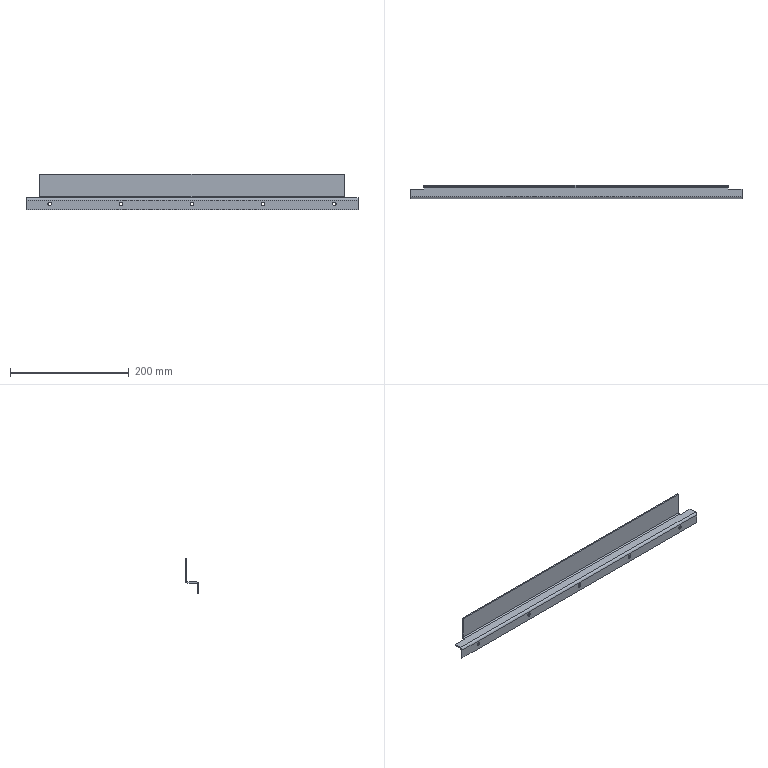Part | NX | features solid 2 | 1 solid | 28 faces | box 560 x 22 x 60 mm | volume 82302 mm3 | plane 14 | cylinder 14 | commonest cylinder face diameters 6 x10 4 x2 8 x2
STEP:
#1=CARTESIAN_POINT('',(1859.9,-1560.,278.));
#2=VERTEX_POINT('',#1);
#3=CARTESIAN_POINT('',(1859.9,-1562.,278.));
#4=VERTEX_POINT('',#3);
#5=CARTESIAN_POINT('',(1859.9,-1578.,278.));
#6=DIRECTION('',(0.,-1.,0.));
#7=VECTOR('',#6,1000.);
#8=LINE('',#5,#7);
#9=EDGE_CURVE('',#2,#4,#8,.T.);
#10=ORIENTED_EDGE('',*,*,#9,.F.);
#11=CARTESIAN_POINT('',(1859.9,-1556.,282.));
#12=VERTEX_POINT('',#11);
#13=CARTESIAN_POINT('',(1859.9,-1560.,282.));
#14=DIRECTION('',(-1.,0.,0.));
#15=DIRECTION('',(0.,0.,-1.));
#16=AXIS2_PLACEMENT_3D('',#13,#14,#15);
#17=CIRCLE('',#16,4.);
#18=EDGE_CURVE('',#12,#2,#17,.T.);
#19=ORIENTED_EDGE('',*,*,#18,.F.);
#20=CARTESIAN_POINT('',(1859.9,-1556.,320.));
#21=VERTEX_POINT('',#20);
#22=CARTESIAN_POINT('',(1859.9,-1556.,280.));
#23=DIRECTION('',(0.,0.,-1.));
#24=VECTOR('',#23,1000.);
#25=LINE('',#22,#24);
#26=EDGE_CURVE('',#21,#12,#25,.T.);
#27=ORIENTED_EDGE('',*,*,#26,.F.);
#28=CARTESIAN_POINT('',(1859.9,-1558.,320.));
#29=VERTEX_POINT('',#28);
#30=CARTESIAN_POINT('',(1859.9,-1558.,320.));
#31=DIRECTION('',(0.,-1.,0.));
#32=VECTOR('',#31,1000.);
#33=LINE('',#30,#32);
#34=EDGE_CURVE('',#21,#29,#33,.T.);
#35=ORIENTED_EDGE('',*,*,#34,.T.);
#36=CARTESIAN_POINT('',(1859.9,-1558.,282.));
#37=VERTEX_POINT('',#36);
#38=CARTESIAN_POINT('',(1859.9,-1558.,280.));
#39=DIRECTION('',(0.,0.,-1.));
#40=VECTOR('',#39,1000.);
#41=LINE('',#38,#40);
#42=EDGE_CURVE('',#29,#37,#41,.T.);
#43=ORIENTED_EDGE('',*,*,#42,.T.);
#44=CARTESIAN_POINT('',(1859.9,-1560.,280.));
#45=VERTEX_POINT('',#44);
#46=CARTESIAN_POINT('',(1859.9,-1560.,282.));
#47=DIRECTION('',(-1.,0.,0.));
#48=DIRECTION('',(0.,0.,-1.));
#49=AXIS2_PLACEMENT_3D('',#46,#47,#48);
#50=CIRCLE('',#49,2.);
#51=EDGE_CURVE('',#37,#45,#50,.T.);
#52=ORIENTED_EDGE('',*,*,#51,.T.);
#53=CARTESIAN_POINT('',(1859.9,-1562.,280.));
#54=VERTEX_POINT('',#53);
#55=CARTESIAN_POINT('',(1859.9,-1578.,280.));
#56=DIRECTION('',(0.,-1.,0.));
#57=VECTOR('',#56,1000.);
#58=LINE('',#55,#57);
#59=EDGE_CURVE('',#45,#54,#58,.T.);
#60=ORIENTED_EDGE('',*,*,#59,.T.);
#61=CARTESIAN_POINT('',(1859.9,-1562.,280.));
#62=DIRECTION('',(0.,0.,1.));
#63=VECTOR('',#62,1000.);
#64=LINE('',#61,#63);
#65=EDGE_CURVE('',#4,#54,#64,.T.);
#66=ORIENTED_EDGE('',*,*,#65,.F.);
#67=EDGE_LOOP('',(#10,#19,#27,#35,#43,#52,#60,#66));
#68=FACE_BOUND('',#67,.T.);
#69=CARTESIAN_POINT('',(1859.9,-1578.,280.));
#70=DIRECTION('',(-1.,0.,0.));
#71=DIRECTION('',(0.,0.,1.));
#72=AXIS2_PLACEMENT_3D('',#69,#70,#71);
#73=PLANE('',#72);
#74=ADVANCED_FACE('',(#68),#73,.F.);
#75=ORIENTED_EDGE('',*,*,#65,.T.);
#76=CARTESIAN_POINT('',(1883.,-1562.,280.));
#77=VERTEX_POINT('',#76);
#78=CARTESIAN_POINT('',(1883.,-1562.,280.));
#79=DIRECTION('',(-1.,0.,0.));
#80=VECTOR('',#79,1000.);
#81=LINE('',#78,#80);
#82=EDGE_CURVE('',#77,#54,#81,.T.);
#83=ORIENTED_EDGE('',*,*,#82,.F.);
#84=CARTESIAN_POINT('',(1883.,-1562.,278.));
#85=VERTEX_POINT('',#84);
#86=CARTESIAN_POINT('',(1883.,-1562.,280.));
#87=DIRECTION('',(0.,0.,1.));
#88=VECTOR('',#87,1000.);
#89=LINE('',#86,#88);
#90=EDGE_CURVE('',#85,#77,#89,.T.);
#91=ORIENTED_EDGE('',*,*,#90,.F.);
#92=CARTESIAN_POINT('',(1883.,-1562.,278.));
#93=DIRECTION('',(-1.,0.,0.));
#94=VECTOR('',#93,1000.);
#95=LINE('',#92,#94);
#96=EDGE_CURVE('',#85,#4,#95,.T.);
#97=ORIENTED_EDGE('',*,*,#96,.T.);
#98=EDGE_LOOP('',(#75,#83,#91,#97));
#99=FACE_BOUND('',#98,.T.);
#100=CARTESIAN_POINT('',(1883.,-1562.,280.));
#101=DIRECTION('',(0.,1.,0.));
#102=DIRECTION('',(0.,0.,-1.));
#103=AXIS2_PLACEMENT_3D('',#100,#101,#102);
#104=PLANE('',#103);
#105=ADVANCED_FACE('',(#99),#104,.T.);
#106=CARTESIAN_POINT('',(1346.1,-1556.,282.));
#107=VERTEX_POINT('',#106);
#108=CARTESIAN_POINT('',(1346.1,-1556.,320.));
#109=VERTEX_POINT('',#108);
#110=CARTESIAN_POINT('',(1346.1,-1556.,280.));
#111=DIRECTION('',(0.,0.,1.));
#112=VECTOR('',#111,1000.);
#113=LINE('',#110,#112);
#114=EDGE_CURVE('',#107,#109,#113,.T.);
#115=ORIENTED_EDGE('',*,*,#114,.F.);
#116=CARTESIAN_POINT('',(1346.1,-1560.,278.));
#117=VERTEX_POINT('',#116);
#118=CARTESIAN_POINT('',(1346.1,-1560.,282.));
#119=DIRECTION('',(1.,0.,0.));
#120=DIRECTION('',(0.,0.,-1.));
#121=AXIS2_PLACEMENT_3D('',#118,#119,#120);
#122=CIRCLE('',#121,4.);
#123=EDGE_CURVE('',#117,#107,#122,.T.);
#124=ORIENTED_EDGE('',*,*,#123,.F.);
#125=CARTESIAN_POINT('',(1346.1,-1562.,278.));
#126=VERTEX_POINT('',#125);
#127=CARTESIAN_POINT('',(1346.1,-1578.,278.));
#128=DIRECTION('',(0.,1.,0.));
#129=VECTOR('',#128,1000.);
#130=LINE('',#127,#129);
#131=EDGE_CURVE('',#126,#117,#130,.T.);
#132=ORIENTED_EDGE('',*,*,#131,.F.);
#133=CARTESIAN_POINT('',(1346.1,-1562.,280.));
#134=VERTEX_POINT('',#133);
#135=CARTESIAN_POINT('',(1346.1,-1562.,280.));
#136=DIRECTION('',(0.,0.,1.));
#137=VECTOR('',#136,1000.);
#138=LINE('',#135,#137);
#139=EDGE_CURVE('',#126,#134,#138,.T.);
#140=ORIENTED_EDGE('',*,*,#139,.T.);
#141=CARTESIAN_POINT('',(1346.1,-1560.,280.));
#142=VERTEX_POINT('',#141);
#143=CARTESIAN_POINT('',(1346.1,-1578.,280.));
#144=DIRECTION('',(0.,1.,0.));
#145=VECTOR('',#144,1000.);
#146=LINE('',#143,#145);
#147=EDGE_CURVE('',#134,#142,#146,.T.);
#148=ORIENTED_EDGE('',*,*,#147,.T.);
#149=CARTESIAN_POINT('',(1346.1,-1558.,282.));
#150=VERTEX_POINT('',#149);
#151=CARTESIAN_POINT('',(1346.1,-1560.,282.));
#152=DIRECTION('',(1.,0.,0.));
#153=DIRECTION('',(0.,0.,1.));
#154=AXIS2_PLACEMENT_3D('',#151,#152,#153);
#155=CIRCLE('',#154,2.);
#156=EDGE_CURVE('',#142,#150,#155,.T.);
#157=ORIENTED_EDGE('',*,*,#156,.T.);
#158=CARTESIAN_POINT('',(1346.1,-1558.,320.));
#159=VERTEX_POINT('',#158);
#160=CARTESIAN_POINT('',(1346.1,-1558.,280.));
#161=DIRECTION('',(0.,0.,1.));
#162=VECTOR('',#161,1000.);
#163=LINE('',#160,#162);
#164=EDGE_CURVE('',#150,#159,#163,.T.);
#165=ORIENTED_EDGE('',*,*,#164,.T.);
#166=CARTESIAN_POINT('',(1346.1,-1558.,320.));
#167=DIRECTION('',(0.,-1.,0.));
#168=VECTOR('',#167,1000.);
#169=LINE('',#166,#168);
#170=EDGE_CURVE('',#109,#159,#169,.T.);
#171=ORIENTED_EDGE('',*,*,#170,.F.);
#172=EDGE_LOOP('',(#115,#124,#132,#140,#148,#157,#165,#171));
#173=FACE_BOUND('',#172,.T.);
#174=CARTESIAN_POINT('',(1346.1,-1558.,280.));
#175=DIRECTION('',(1.,0.,0.));
#176=DIRECTION('',(0.,0.,1.));
#177=AXIS2_PLACEMENT_3D('',#174,#175,#176);
#178=PLANE('',#177);
#179=ADVANCED_FACE('',(#173),#178,.F.);
#180=CARTESIAN_POINT('',(1323.,-1562.,278.));
#181=VERTEX_POINT('',#180);
#182=CARTESIAN_POINT('',(1323.,-1562.,280.));
#183=VERTEX_POINT('',#182);
#184=CARTESIAN_POINT('',(1323.,-1562.,280.));
#185=DIRECTION('',(0.,0.,1.));
#186=VECTOR('',#185,1000.);
#187=LINE('',#184,#186);
#188=EDGE_CURVE('',#181,#183,#187,.T.);
#189=ORIENTED_EDGE('',*,*,#188,.T.);
#190=CARTESIAN_POINT('',(1883.,-1562.,280.));
#191=DIRECTION('',(-1.,0.,0.));
#192=VECTOR('',#191,1000.);
#193=LINE('',#190,#192);
#194=EDGE_CURVE('',#134,#183,#193,.T.);
#195=ORIENTED_EDGE('',*,*,#194,.F.);
#196=ORIENTED_EDGE('',*,*,#139,.F.);
#197=CARTESIAN_POINT('',(1883.,-1562.,278.));
#198=DIRECTION('',(-1.,0.,0.));
#199=VECTOR('',#198,1000.);
#200=LINE('',#197,#199);
#201=EDGE_CURVE('',#126,#181,#200,.T.);
#202=ORIENTED_EDGE('',*,*,#201,.T.);
#203=EDGE_LOOP('',(#189,#195,#196,#202));
#204=FACE_BOUND('',#203,.T.);
#205=CARTESIAN_POINT('',(1883.,-1562.,280.));
#206=DIRECTION('',(0.,1.,0.));
#207=DIRECTION('',(0.,0.,-1.));
#208=AXIS2_PLACEMENT_3D('',#205,#206,#207);
#209=PLANE('',#208);
#210=ADVANCED_FACE('',(#204),#209,.T.);
#211=CARTESIAN_POINT('',(1603.,-1578.,267.));
#212=VERTEX_POINT('',#211);
#213=CARTESIAN_POINT('',(1603.,-1576.,267.));
#214=VERTEX_POINT('',#213);
#215=CARTESIAN_POINT('',(1603.,-2139.635,267.));
#216=DIRECTION('',(0.,1.,0.));
#217=VECTOR('',#216,1000.);
#218=LINE('',#215,#217);
#219=EDGE_CURVE('',#212,#214,#218,.T.);
#220=ORIENTED_EDGE('',*,*,#219,.F.);
#221=CARTESIAN_POINT('',(1603.,-1578.,273.));
#222=VERTEX_POINT('',#221);
#223=CARTESIAN_POINT('',(1603.,-1578.,270.));
#224=DIRECTION('',(0.,-1.,0.));
#225=DIRECTION('',(0.,0.,-1.));
#226=AXIS2_PLACEMENT_3D('',#223,#224,#225);
#227=CIRCLE('',#226,3.);
#228=EDGE_CURVE('',#212,#222,#227,.T.);
#229=ORIENTED_EDGE('',*,*,#228,.T.);
#230=CARTESIAN_POINT('',(1603.,-1576.,273.));
#231=VERTEX_POINT('',#230);
#232=CARTESIAN_POINT('',(1603.,-2139.635,273.));
#233=DIRECTION('',(0.,1.,0.));
#234=VECTOR('',#233,1000.);
#235=LINE('',#232,#234);
#236=EDGE_CURVE('',#231,#222,#235,.F.);
#237=ORIENTED_EDGE('',*,*,#236,.F.);
#238=CARTESIAN_POINT('',(1603.,-1576.,270.));
#239=DIRECTION('',(0.,1.,0.));
#240=DIRECTION('',(-1.,0.,0.));
#241=AXIS2_PLACEMENT_3D('',#238,#239,#240);
#242=CIRCLE('',#241,3.);
#243=EDGE_CURVE('',#231,#214,#242,.T.);
#244=ORIENTED_EDGE('',*,*,#243,.T.);
#245=EDGE_LOOP('',(#220,#229,#237,#244));
#246=FACE_BOUND('',#245,.T.);
#247=CARTESIAN_POINT('',(1603.,-2139.635,270.));
#248=DIRECTION('',(0.,1.,0.));
#249=DIRECTION('',(0.,0.,1.));
#250=AXIS2_PLACEMENT_3D('',#247,#248,#249);
#251=CYLINDRICAL_SURFACE('',#250,3.);
#252=ADVANCED_FACE('',(#246),#251,.F.);
#253=CARTESIAN_POINT('',(1843.,-1578.,267.));
#254=VERTEX_POINT('',#253);
#255=CARTESIAN_POINT('',(1843.,-1576.,267.));
#256=VERTEX_POINT('',#255);
#257=CARTESIAN_POINT('',(1843.,-2139.635,267.));
#258=DIRECTION('',(0.,1.,0.));
#259=VECTOR('',#258,1000.);
#260=LINE('',#257,#259);
#261=EDGE_CURVE('',#254,#256,#260,.T.);
#262=ORIENTED_EDGE('',*,*,#261,.F.);
#263=CARTESIAN_POINT('',(1843.,-1578.,273.));
#264=VERTEX_POINT('',#263);
#265=CARTESIAN_POINT('',(1843.,-1578.,270.));
#266=DIRECTION('',(0.,-1.,0.));
#267=DIRECTION('',(0.,0.,-1.));
#268=AXIS2_PLACEMENT_3D('',#265,#266,#267);
#269=CIRCLE('',#268,3.);
#270=EDGE_CURVE('',#254,#264,#269,.T.);
#271=ORIENTED_EDGE('',*,*,#270,.T.);
#272=CARTESIAN_POINT('',(1843.,-1576.,273.));
#273=VERTEX_POINT('',#272);
#274=CARTESIAN_POINT('',(1843.,-2139.635,273.));
#275=DIRECTION('',(0.,1.,0.));
#276=VECTOR('',#275,1000.);
#277=LINE('',#274,#276);
#278=EDGE_CURVE('',#273,#264,#277,.F.);
#279=ORIENTED_EDGE('',*,*,#278,.F.);
#280=CARTESIAN_POINT('',(1843.,-1576.,270.));
#281=DIRECTION('',(0.,1.,0.));
#282=DIRECTION('',(-1.,0.,0.));
#283=AXIS2_PLACEMENT_3D('',#280,#281,#282);
#284=CIRCLE('',#283,3.);
#285=EDGE_CURVE('',#273,#256,#284,.T.);
#286=ORIENTED_EDGE('',*,*,#285,.T.);
#287=EDGE_LOOP('',(#262,#271,#279,#286));
#288=FACE_BOUND('',#287,.T.);
#289=CARTESIAN_POINT('',(1843.,-2139.635,270.));
#290=DIRECTION('',(0.,1.,0.));
#291=DIRECTION('',(0.,0.,1.));
#292=AXIS2_PLACEMENT_3D('',#289,#290,#291);
#293=CYLINDRICAL_SURFACE('',#292,3.);
#294=ADVANCED_FACE('',(#288),#293,.F.);
#295=CARTESIAN_POINT('',(1723.,-1578.,267.));
#296=VERTEX_POINT('',#295);
#297=CARTESIAN_POINT('',(1723.,-1576.,267.));
#298=VERTEX_POINT('',#297);
#299=CARTESIAN_POINT('',(1723.,-2139.635,267.));
#300=DIRECTION('',(0.,1.,0.));
#301=VECTOR('',#300,1000.);
#302=LINE('',#299,#301);
#303=EDGE_CURVE('',#296,#298,#302,.T.);
#304=ORIENTED_EDGE('',*,*,#303,.F.);
#305=CARTESIAN_POINT('',(1723.,-1578.,273.));
#306=VERTEX_POINT('',#305);
#307=CARTESIAN_POINT('',(1723.,-1578.,270.));
#308=DIRECTION('',(0.,-1.,0.));
#309=DIRECTION('',(0.,0.,-1.));
#310=AXIS2_PLACEMENT_3D('',#307,#308,#309);
#311=CIRCLE('',#310,3.);
#312=EDGE_CURVE('',#296,#306,#311,.T.);
#313=ORIENTED_EDGE('',*,*,#312,.T.);
#314=CARTESIAN_POINT('',(1723.,-1576.,273.));
#315=VERTEX_POINT('',#314);
#316=CARTESIAN_POINT('',(1723.,-2139.635,273.));
#317=DIRECTION('',(0.,1.,0.));
#318=VECTOR('',#317,1000.);
#319=LINE('',#316,#318);
#320=EDGE_CURVE('',#315,#306,#319,.F.);
#321=ORIENTED_EDGE('',*,*,#320,.F.);
#322=CARTESIAN_POINT('',(1723.,-1576.,270.));
#323=DIRECTION('',(0.,1.,0.));
#324=DIRECTION('',(-1.,0.,0.));
#325=AXIS2_PLACEMENT_3D('',#322,#323,#324);
#326=CIRCLE('',#325,3.);
#327=EDGE_CURVE('',#315,#298,#326,.T.);
#328=ORIENTED_EDGE('',*,*,#327,.T.);
#329=EDGE_LOOP('',(#304,#313,#321,#328));
#330=FACE_BOUND('',#329,.T.);
#331=CARTESIAN_POINT('',(1723.,-2139.635,270.));
#332=DIRECTION('',(0.,1.,0.));
#333=DIRECTION('',(0.,0.,1.));
#334=AXIS2_PLACEMENT_3D('',#331,#332,#333);
#335=CYLINDRICAL_SURFACE('',#334,3.);
#336=ADVANCED_FACE('',(#330),#335,.F.);
#337=CARTESIAN_POINT('',(1363.,-1576.,267.));
#338=VERTEX_POINT('',#337);
#339=CARTESIAN_POINT('',(1363.,-1578.,267.));
#340=VERTEX_POINT('',#339);
#341=CARTESIAN_POINT('',(1363.,-2139.635,267.));
#342=DIRECTION('',(0.,1.,0.));
#343=VECTOR('',#342,1000.);
#344=LINE('',#341,#343);
#345=EDGE_CURVE('',#338,#340,#344,.F.);
#346=ORIENTED_EDGE('',*,*,#345,.T.);
#347=CARTESIAN_POINT('',(1363.,-1578.,273.));
#348=VERTEX_POINT('',#347);
#349=CARTESIAN_POINT('',(1363.,-1578.,270.));
#350=DIRECTION('',(0.,-1.,0.));
#351=DIRECTION('',(0.,0.,-1.));
#352=AXIS2_PLACEMENT_3D('',#349,#350,#351);
#353=CIRCLE('',#352,3.);
#354=EDGE_CURVE('',#340,#348,#353,.T.);
#355=ORIENTED_EDGE('',*,*,#354,.T.);
#356=CARTESIAN_POINT('',(1363.,-1576.,273.));
#357=VERTEX_POINT('',#356);
#358=CARTESIAN_POINT('',(1363.,-2139.635,273.));
#359=DIRECTION('',(0.,1.,0.));
#360=VECTOR('',#359,1000.);
#361=LINE('',#358,#360);
#362=EDGE_CURVE('',#348,#357,#361,.T.);
#363=ORIENTED_EDGE('',*,*,#362,.T.);
#364=CARTESIAN_POINT('',(1363.,-1576.,270.));
#365=DIRECTION('',(0.,1.,0.));
#366=DIRECTION('',(-1.,0.,0.));
#367=AXIS2_PLACEMENT_3D('',#364,#365,#366);
#368=CIRCLE('',#367,3.);
#369=EDGE_CURVE('',#357,#338,#368,.T.);
#370=ORIENTED_EDGE('',*,*,#369,.T.);
#371=EDGE_LOOP('',(#346,#355,#363,#370));
#372=FACE_BOUND('',#371,.T.);
#373=CARTESIAN_POINT('',(1363.,-2139.635,270.));
#374=DIRECTION('',(0.,1.,0.));
#375=DIRECTION('',(0.,0.,1.));
#376=AXIS2_PLACEMENT_3D('',#373,#374,#375);
#377=CYLINDRICAL_SURFACE('',#376,3.);
#378=ADVANCED_FACE('',(#372),#377,.F.);
#379=CARTESIAN_POINT('',(1483.,-1576.,267.));
#380=VERTEX_POINT('',#379);
#381=CARTESIAN_POINT('',(1483.,-1578.,267.));
#382=VERTEX_POINT('',#381);
#383=CARTESIAN_POINT('',(1483.,-2139.635,267.));
#384=DIRECTION('',(0.,1.,0.));
#385=VECTOR('',#384,1000.);
#386=LINE('',#383,#385);
#387=EDGE_CURVE('',#380,#382,#386,.F.);
#388=ORIENTED_EDGE('',*,*,#387,.T.);
#389=CARTESIAN_POINT('',(1483.,-1578.,273.));
#390=VERTEX_POINT('',#389);
#391=CARTESIAN_POINT('',(1483.,-1578.,270.));
#392=DIRECTION('',(0.,-1.,0.));
#393=DIRECTION('',(0.,0.,-1.));
#394=AXIS2_PLACEMENT_3D('',#391,#392,#393);
#395=CIRCLE('',#394,3.);
#396=EDGE_CURVE('',#382,#390,#395,.T.);
#397=ORIENTED_EDGE('',*,*,#396,.T.);
#398=CARTESIAN_POINT('',(1483.,-1576.,273.));
#399=VERTEX_POINT('',#398);
#400=CARTESIAN_POINT('',(1483.,-2139.635,273.));
#401=DIRECTION('',(0.,1.,0.));
#402=VECTOR('',#401,1000.);
#403=LINE('',#400,#402);
#404=EDGE_CURVE('',#390,#399,#403,.T.);
#405=ORIENTED_EDGE('',*,*,#404,.T.);
#406=CARTESIAN_POINT('',(1483.,-1576.,270.));
#407=DIRECTION('',(0.,1.,0.));
#408=DIRECTION('',(-1.,0.,0.));
#409=AXIS2_PLACEMENT_3D('',#406,#407,#408);
#410=CIRCLE('',#409,3.);
#411=EDGE_CURVE('',#399,#380,#410,.T.);
#412=ORIENTED_EDGE('',*,*,#411,.T.);
#413=EDGE_LOOP('',(#388,#397,#405,#412));
#414=FACE_BOUND('',#413,.T.);
#415=CARTESIAN_POINT('',(1483.,-2139.635,270.));
#416=DIRECTION('',(0.,1.,0.));
#417=DIRECTION('',(0.,0.,1.));
#418=AXIS2_PLACEMENT_3D('',#415,#416,#417);
#419=CYLINDRICAL_SURFACE('',#418,3.);
#420=ADVANCED_FACE('',(#414),#419,.F.);
#421=CARTESIAN_POINT('',(1883.,-1556.,320.));
#422=DIRECTION('',(-1.,0.,0.));
#423=VECTOR('',#422,1000.);
#424=LINE('',#421,#423);
#425=EDGE_CURVE('',#21,#109,#424,.T.);
#426=ORIENTED_EDGE('',*,*,#425,.F.);
#427=ORIENTED_EDGE('',*,*,#26,.T.);
#428=CARTESIAN_POINT('',(1883.,-1556.,282.));
#429=DIRECTION('',(-1.,0.,0.));
#430=VECTOR('',#429,1000.);
#431=LINE('',#428,#430);
#432=EDGE_CURVE('',#12,#107,#431,.T.);
#433=ORIENTED_EDGE('',*,*,#432,.T.);
#434=ORIENTED_EDGE('',*,*,#114,.T.);
#435=EDGE_LOOP('',(#426,#427,#433,#434));
#436=FACE_BOUND('',#435,.T.);
#437=CARTESIAN_POINT('',(1883.,-1556.,280.));
#438=DIRECTION('',(0.,-1.,0.));
#439=DIRECTION('',(-1.,0.,0.));
#440=AXIS2_PLACEMENT_3D('',#437,#438,#439);
#441=PLANE('',#440);
#442=ADVANCED_FACE('',(#436),#441,.F.);
#443=ORIENTED_EDGE('',*,*,#432,.F.);
#444=ORIENTED_EDGE('',*,*,#18,.T.);
#445=CARTESIAN_POINT('',(1883.,-1560.,278.));
#446=DIRECTION('',(-1.,0.,0.));
#447=VECTOR('',#446,1000.);
#448=LINE('',#445,#447);
#449=EDGE_CURVE('',#2,#117,#448,.T.);
#450=ORIENTED_EDGE('',*,*,#449,.T.);
#451=ORIENTED_EDGE('',*,*,#123,.T.);
#452=EDGE_LOOP('',(#443,#444,#450,#451));
#453=FACE_BOUND('',#452,.T.);
#454=CARTESIAN_POINT('',(1883.,-1560.,282.));
#455=DIRECTION('',(-1.,0.,0.));
#456=DIRECTION('',(0.,0.,-1.));
#457=AXIS2_PLACEMENT_3D('',#454,#455,#456);
#458=CYLINDRICAL_SURFACE('',#457,4.);
#459=ADVANCED_FACE('',(#453),#458,.T.);
#460=ORIENTED_EDGE('',*,*,#9,.T.);
#461=ORIENTED_EDGE('',*,*,#96,.F.);
#462=CARTESIAN_POINT('',(1883.,-1574.,278.));
#463=VERTEX_POINT('',#462);
#464=CARTESIAN_POINT('',(1883.,-1578.,278.));
#465=DIRECTION('',(0.,1.,0.));
#466=VECTOR('',#465,1000.);
#467=LINE('',#464,#466);
#468=EDGE_CURVE('',#463,#85,#467,.T.);
#469=ORIENTED_EDGE('',*,*,#468,.F.);
#470=CARTESIAN_POINT('',(1323.,-1574.,278.));
#471=VERTEX_POINT('',#470);
#472=CARTESIAN_POINT('',(1883.,-1574.,278.));
#473=DIRECTION('',(-1.,0.,0.));
#474=VECTOR('',#473,1000.);
#475=LINE('',#472,#474);
#476=EDGE_CURVE('',#463,#471,#475,.T.);
#477=ORIENTED_EDGE('',*,*,#476,.T.);
#478=CARTESIAN_POINT('',(1323.,-1578.,278.));
#479=DIRECTION('',(0.,1.,0.));
#480=VECTOR('',#479,1000.);
#481=LINE('',#478,#480);
#482=EDGE_CURVE('',#471,#181,#481,.T.);
#483=ORIENTED_EDGE('',*,*,#482,.T.);
#484=ORIENTED_EDGE('',*,*,#201,.F.);
#485=ORIENTED_EDGE('',*,*,#131,.T.);
#486=ORIENTED_EDGE('',*,*,#449,.F.);
#487=EDGE_LOOP('',(#460,#461,#469,#477,#483,#484,#485,#486));
#488=FACE_BOUND('',#487,.T.);
#489=CARTESIAN_POINT('',(1883.,-1578.,278.));
#490=DIRECTION('',(0.,0.,1.));
#491=DIRECTION('',(0.,-1.,0.));
#492=AXIS2_PLACEMENT_3D('',#489,#490,#491);
#493=PLANE('',#492);
#494=ADVANCED_FACE('',(#488),#493,.F.);
#495=CARTESIAN_POINT('',(1323.,-1576.,276.));
#496=VERTEX_POINT('',#495);
#497=CARTESIAN_POINT('',(1323.,-1574.,276.));
#498=DIRECTION('',(-1.,0.,0.));
#499=DIRECTION('',(0.,0.,-1.));
#500=AXIS2_PLACEMENT_3D('',#497,#498,#499);
#501=CIRCLE('',#500,2.);
#502=EDGE_CURVE('',#496,#471,#501,.T.);
#503=ORIENTED_EDGE('',*,*,#502,.T.);
#504=ORIENTED_EDGE('',*,*,#476,.F.);
#505=CARTESIAN_POINT('',(1883.,-1576.,276.));
#506=VERTEX_POINT('',#505);
#507=CARTESIAN_POINT('',(1883.,-1574.,276.));
#508=DIRECTION('',(-1.,0.,0.));
#509=DIRECTION('',(0.,0.,-1.));
#510=AXIS2_PLACEMENT_3D('',#507,#508,#509);
#511=CIRCLE('',#510,2.);
#512=EDGE_CURVE('',#506,#463,#511,.T.);
#513=ORIENTED_EDGE('',*,*,#512,.F.);
#514=CARTESIAN_POINT('',(1883.,-1576.,276.));
#515=DIRECTION('',(-1.,0.,0.));
#516=VECTOR('',#515,1000.);
#517=LINE('',#514,#516);
#518=EDGE_CURVE('',#506,#496,#517,.T.);
#519=ORIENTED_EDGE('',*,*,#518,.T.);
#520=EDGE_LOOP('',(#503,#504,#513,#519));
#521=FACE_BOUND('',#520,.T.);
#522=CARTESIAN_POINT('',(1883.,-1574.,276.));
#523=DIRECTION('',(-1.,0.,0.));
#524=DIRECTION('',(0.,0.,-1.));
#525=AXIS2_PLACEMENT_3D('',#522,#523,#524);
#526=CYLINDRICAL_SURFACE('',#525,2.);
#527=ADVANCED_FACE('',(#521),#526,.F.);
#528=ORIENTED_EDGE('',*,*,#411,.F.);
#529=CARTESIAN_POINT('',(1483.,-1576.,270.));
#530=DIRECTION('',(0.,1.,0.));
#531=DIRECTION('',(-1.,0.,0.));
#532=AXIS2_PLACEMENT_3D('',#529,#530,#531);
#533=CIRCLE('',#532,3.);
#534=EDGE_CURVE('',#380,#399,#533,.T.);
#535=ORIENTED_EDGE('',*,*,#534,.F.);
#536=EDGE_LOOP('',(#528,#535));
#537=FACE_BOUND('',#536,.T.);
#538=ORIENTED_EDGE('',*,*,#369,.F.);
#539=CARTESIAN_POINT('',(1363.,-1576.,270.));
#540=DIRECTION('',(0.,1.,0.));
#541=DIRECTION('',(-1.,0.,0.));
#542=AXIS2_PLACEMENT_3D('',#539,#540,#541);
#543=CIRCLE('',#542,3.);
#544=EDGE_CURVE('',#338,#357,#543,.T.);
#545=ORIENTED_EDGE('',*,*,#544,.F.);
#546=EDGE_LOOP('',(#538,#545));
#547=FACE_BOUND('',#546,.T.);
#548=ORIENTED_EDGE('',*,*,#327,.F.);
#549=CARTESIAN_POINT('',(1723.,-1576.,270.));
#550=DIRECTION('',(0.,1.,0.));
#551=DIRECTION('',(-1.,0.,0.));
#552=AXIS2_PLACEMENT_3D('',#549,#550,#551);
#553=CIRCLE('',#552,3.);
#554=EDGE_CURVE('',#298,#315,#553,.T.);
#555=ORIENTED_EDGE('',*,*,#554,.F.);
#556=EDGE_LOOP('',(#548,#555));
#557=FACE_BOUND('',#556,.T.);
#558=ORIENTED_EDGE('',*,*,#285,.F.);
#559=CARTESIAN_POINT('',(1843.,-1576.,270.));
#560=DIRECTION('',(0.,1.,0.));
#561=DIRECTION('',(-1.,0.,0.));
#562=AXIS2_PLACEMENT_3D('',#559,#560,#561);
#563=CIRCLE('',#562,3.);
#564=EDGE_CURVE('',#256,#273,#563,.T.);
#565=ORIENTED_EDGE('',*,*,#564,.F.);
#566=EDGE_LOOP('',(#558,#565));
#567=FACE_BOUND('',#566,.T.);
#568=ORIENTED_EDGE('',*,*,#243,.F.);
#569=CARTESIAN_POINT('',(1603.,-1576.,270.));
#570=DIRECTION('',(0.,1.,0.));
#571=DIRECTION('',(-1.,0.,0.));
#572=AXIS2_PLACEMENT_3D('',#569,#570,#571);
#573=CIRCLE('',#572,3.);
#574=EDGE_CURVE('',#214,#231,#573,.T.);
#575=ORIENTED_EDGE('',*,*,#574,.F.);
#576=EDGE_LOOP('',(#568,#575));
#577=FACE_BOUND('',#576,.T.);
#578=CARTESIAN_POINT('',(1323.,-1576.,260.));
#579=VERTEX_POINT('',#578);
#580=CARTESIAN_POINT('',(1323.,-1576.,260.));
#581=DIRECTION('',(0.,0.,1.));
#582=VECTOR('',#581,1000.);
#583=LINE('',#580,#582);
#584=EDGE_CURVE('',#579,#496,#583,.T.);
#585=ORIENTED_EDGE('',*,*,#584,.T.);
#586=ORIENTED_EDGE('',*,*,#518,.F.);
#587=CARTESIAN_POINT('',(1883.,-1576.,260.));
#588=VERTEX_POINT('',#587);
#589=CARTESIAN_POINT('',(1883.,-1576.,260.));
#590=DIRECTION('',(0.,0.,1.));
#591=VECTOR('',#590,1000.);
#592=LINE('',#589,#591);
#593=EDGE_CURVE('',#588,#506,#592,.T.);
#594=ORIENTED_EDGE('',*,*,#593,.F.);
#595=CARTESIAN_POINT('',(1883.,-1576.,260.));
#596=DIRECTION('',(-1.,0.,0.));
#597=VECTOR('',#596,1000.);
#598=LINE('',#595,#597);
#599=EDGE_CURVE('',#588,#579,#598,.T.);
#600=ORIENTED_EDGE('',*,*,#599,.T.);
#601=EDGE_LOOP('',(#585,#586,#594,#600));
#602=FACE_BOUND('',#601,.T.);
#603=CARTESIAN_POINT('',(1883.,-1576.,260.));
#604=DIRECTION('',(0.,-1.,0.));
#605=DIRECTION('',(-1.,0.,0.));
#606=AXIS2_PLACEMENT_3D('',#603,#604,#605);
#607=PLANE('',#606);
#608=ADVANCED_FACE('',(#537,#547,#557,#567,#577,#602),#607,.F.);
#609=ORIENTED_EDGE('',*,*,#42,.F.);
#610=CARTESIAN_POINT('',(1883.,-1558.,320.));
#611=DIRECTION('',(-1.,0.,0.));
#612=VECTOR('',#611,1000.);
#613=LINE('',#610,#612);
#614=EDGE_CURVE('',#29,#159,#613,.T.);
#615=ORIENTED_EDGE('',*,*,#614,.T.);
#616=ORIENTED_EDGE('',*,*,#164,.F.);
#617=CARTESIAN_POINT('',(1883.,-1558.,282.));
#618=DIRECTION('',(-1.,0.,0.));
#619=VECTOR('',#618,1000.);
#620=LINE('',#617,#619);
#621=EDGE_CURVE('',#37,#150,#620,.T.);
#622=ORIENTED_EDGE('',*,*,#621,.F.);
#623=EDGE_LOOP('',(#609,#615,#616,#622));
#624=FACE_BOUND('',#623,.T.);
#625=CARTESIAN_POINT('',(1883.,-1558.,280.));
#626=DIRECTION('',(0.,-1.,0.));
#627=DIRECTION('',(-1.,0.,0.));
#628=AXIS2_PLACEMENT_3D('',#625,#626,#627);
#629=PLANE('',#628);
#630=ADVANCED_FACE('',(#624),#629,.T.);
#631=ORIENTED_EDGE('',*,*,#51,.F.);
#632=ORIENTED_EDGE('',*,*,#621,.T.);
#633=ORIENTED_EDGE('',*,*,#156,.F.);
#634=CARTESIAN_POINT('',(1883.,-1560.,280.));
#635=DIRECTION('',(-1.,0.,0.));
#636=VECTOR('',#635,1000.);
#637=LINE('',#634,#636);
#638=EDGE_CURVE('',#45,#142,#637,.T.);
#639=ORIENTED_EDGE('',*,*,#638,.F.);
#640=EDGE_LOOP('',(#631,#632,#633,#639));
#641=FACE_BOUND('',#640,.T.);
#642=CARTESIAN_POINT('',(1883.,-1560.,282.));
#643=DIRECTION('',(-1.,0.,0.));
#644=DIRECTION('',(0.,0.,-1.));
#645=AXIS2_PLACEMENT_3D('',#642,#643,#644);
#646=CYLINDRICAL_SURFACE('',#645,2.);
#647=ADVANCED_FACE('',(#641),#646,.F.);
#648=ORIENTED_EDGE('',*,*,#82,.T.);
#649=ORIENTED_EDGE('',*,*,#59,.F.);
#650=ORIENTED_EDGE('',*,*,#638,.T.);
#651=ORIENTED_EDGE('',*,*,#147,.F.);
#652=ORIENTED_EDGE('',*,*,#194,.T.);
#653=CARTESIAN_POINT('',(1323.,-1574.,280.));
#654=VERTEX_POINT('',#653);
#655=CARTESIAN_POINT('',(1323.,-1578.,280.));
#656=DIRECTION('',(0.,1.,0.));
#657=VECTOR('',#656,1000.);
#658=LINE('',#655,#657);
#659=EDGE_CURVE('',#654,#183,#658,.T.);
#660=ORIENTED_EDGE('',*,*,#659,.F.);
#661=CARTESIAN_POINT('',(1883.,-1574.,280.));
#662=VERTEX_POINT('',#661);
#663=CARTESIAN_POINT('',(1883.,-1574.,280.));
#664=DIRECTION('',(-1.,0.,0.));
#665=VECTOR('',#664,1000.);
#666=LINE('',#663,#665);
#667=EDGE_CURVE('',#662,#654,#666,.T.);
#668=ORIENTED_EDGE('',*,*,#667,.F.);
#669=CARTESIAN_POINT('',(1883.,-1578.,280.));
#670=DIRECTION('',(0.,1.,0.));
#671=VECTOR('',#670,1000.);
#672=LINE('',#669,#671);
#673=EDGE_CURVE('',#662,#77,#672,.T.);
#674=ORIENTED_EDGE('',*,*,#673,.T.);
#675=EDGE_LOOP('',(#648,#649,#650,#651,#652,#660,#668,#674));
#676=FACE_BOUND('',#675,.T.);
#677=CARTESIAN_POINT('',(1883.,-1578.,280.));
#678=DIRECTION('',(0.,0.,1.));
#679=DIRECTION('',(0.,-1.,0.));
#680=AXIS2_PLACEMENT_3D('',#677,#678,#679);
#681=PLANE('',#680);
#682=ADVANCED_FACE('',(#676),#681,.T.);
#683=CARTESIAN_POINT('',(1323.,-1578.,276.));
#684=VERTEX_POINT('',#683);
#685=CARTESIAN_POINT('',(1323.,-1574.,276.));
#686=DIRECTION('',(-1.,0.,0.));
#687=DIRECTION('',(0.,0.,1.));
#688=AXIS2_PLACEMENT_3D('',#685,#686,#687);
#689=CIRCLE('',#688,4.);
#690=EDGE_CURVE('',#684,#654,#689,.T.);
#691=ORIENTED_EDGE('',*,*,#690,.F.);
#692=CARTESIAN_POINT('',(1883.,-1578.,276.));
#693=VERTEX_POINT('',#692);
#694=CARTESIAN_POINT('',(1883.,-1578.,276.));
#695=DIRECTION('',(-1.,0.,0.));
#696=VECTOR('',#695,1000.);
#697=LINE('',#694,#696);
#698=EDGE_CURVE('',#693,#684,#697,.T.);
#699=ORIENTED_EDGE('',*,*,#698,.F.);
#700=CARTESIAN_POINT('',(1883.,-1574.,276.));
#701=DIRECTION('',(-1.,0.,0.));
#702=DIRECTION('',(0.,0.,1.));
#703=AXIS2_PLACEMENT_3D('',#700,#701,#702);
#704=CIRCLE('',#703,4.);
#705=EDGE_CURVE('',#693,#662,#704,.T.);
#706=ORIENTED_EDGE('',*,*,#705,.T.);
#707=ORIENTED_EDGE('',*,*,#667,.T.);
#708=EDGE_LOOP('',(#691,#699,#706,#707));
#709=FACE_BOUND('',#708,.T.);
#710=CARTESIAN_POINT('',(1883.,-1574.,276.));
#711=DIRECTION('',(-1.,0.,0.));
#712=DIRECTION('',(0.,0.,-1.));
#713=AXIS2_PLACEMENT_3D('',#710,#711,#712);
#714=CYLINDRICAL_SURFACE('',#713,4.);
#715=ADVANCED_FACE('',(#709),#714,.T.);
#716=CARTESIAN_POINT('',(1483.,-1578.,270.));
#717=DIRECTION('',(0.,-1.,0.));
#718=DIRECTION('',(0.,0.,-1.));
#719=AXIS2_PLACEMENT_3D('',#716,#717,#718);
#720=CIRCLE('',#719,3.);
#721=EDGE_CURVE('',#390,#382,#720,.T.);
#722=ORIENTED_EDGE('',*,*,#721,.F.);
#723=ORIENTED_EDGE('',*,*,#396,.F.);
#724=EDGE_LOOP('',(#722,#723));
#725=FACE_BOUND('',#724,.T.);
#726=CARTESIAN_POINT('',(1363.,-1578.,270.));
#727=DIRECTION('',(0.,-1.,0.));
#728=DIRECTION('',(0.,0.,-1.));
#729=AXIS2_PLACEMENT_3D('',#726,#727,#728);
#730=CIRCLE('',#729,3.);
#731=EDGE_CURVE('',#348,#340,#730,.T.);
#732=ORIENTED_EDGE('',*,*,#731,.F.);
#733=ORIENTED_EDGE('',*,*,#354,.F.);
#734=EDGE_LOOP('',(#732,#733));
#735=FACE_BOUND('',#734,.T.);
#736=CARTESIAN_POINT('',(1723.,-1578.,270.));
#737=DIRECTION('',(0.,-1.,0.));
#738=DIRECTION('',(0.,0.,-1.));
#739=AXIS2_PLACEMENT_3D('',#736,#737,#738);
#740=CIRCLE('',#739,3.);
#741=EDGE_CURVE('',#306,#296,#740,.T.);
#742=ORIENTED_EDGE('',*,*,#741,.F.);
#743=ORIENTED_EDGE('',*,*,#312,.F.);
#744=EDGE_LOOP('',(#742,#743));
#745=FACE_BOUND('',#744,.T.);
#746=CARTESIAN_POINT('',(1843.,-1578.,270.));
#747=DIRECTION('',(0.,-1.,0.));
#748=DIRECTION('',(0.,0.,-1.));
#749=AXIS2_PLACEMENT_3D('',#746,#747,#748);
#750=CIRCLE('',#749,3.);
#751=EDGE_CURVE('',#264,#254,#750,.T.);
#752=ORIENTED_EDGE('',*,*,#751,.F.);
#753=ORIENTED_EDGE('',*,*,#270,.F.);
#754=EDGE_LOOP('',(#752,#753));
#755=FACE_BOUND('',#754,.T.);
#756=CARTESIAN_POINT('',(1603.,-1578.,270.));
#757=DIRECTION('',(0.,-1.,0.));
#758=DIRECTION('',(0.,0.,-1.));
#759=AXIS2_PLACEMENT_3D('',#756,#757,#758);
#760=CIRCLE('',#759,3.);
#761=EDGE_CURVE('',#222,#212,#760,.T.);
#762=ORIENTED_EDGE('',*,*,#761,.F.);
#763=ORIENTED_EDGE('',*,*,#228,.F.);
#764=EDGE_LOOP('',(#762,#763));
#765=FACE_BOUND('',#764,.T.);
#766=CARTESIAN_POINT('',(1323.,-1578.,260.));
#767=VERTEX_POINT('',#766);
#768=CARTESIAN_POINT('',(1323.,-1578.,260.));
#769=DIRECTION('',(0.,0.,1.));
#770=VECTOR('',#769,1000.);
#771=LINE('',#768,#770);
#772=EDGE_CURVE('',#767,#684,#771,.T.);
#773=ORIENTED_EDGE('',*,*,#772,.F.);
#774=CARTESIAN_POINT('',(1883.,-1578.,260.));
#775=VERTEX_POINT('',#774);
#776=CARTESIAN_POINT('',(1883.,-1578.,260.));
#777=DIRECTION('',(-1.,0.,0.));
#778=VECTOR('',#777,1000.);
#779=LINE('',#776,#778);
#780=EDGE_CURVE('',#775,#767,#779,.T.);
#781=ORIENTED_EDGE('',*,*,#780,.F.);
#782=CARTESIAN_POINT('',(1883.,-1578.,260.));
#783=DIRECTION('',(0.,0.,1.));
#784=VECTOR('',#783,1000.);
#785=LINE('',#782,#784);
#786=EDGE_CURVE('',#775,#693,#785,.T.);
#787=ORIENTED_EDGE('',*,*,#786,.T.);
#788=ORIENTED_EDGE('',*,*,#698,.T.);
#789=EDGE_LOOP('',(#773,#781,#787,#788));
#790=FACE_BOUND('',#789,.T.);
#791=CARTESIAN_POINT('',(1883.,-1578.,260.));
#792=DIRECTION('',(0.,-1.,0.));
#793=DIRECTION('',(-1.,0.,0.));
#794=AXIS2_PLACEMENT_3D('',#791,#792,#793);
#795=PLANE('',#794);
#796=ADVANCED_FACE('',(#725,#735,#745,#755,#765,#790),#795,.T.);
#797=ORIENTED_EDGE('',*,*,#599,.F.);
#798=CARTESIAN_POINT('',(1883.,-1578.,260.));
#799=DIRECTION('',(0.,-1.,0.));
#800=VECTOR('',#799,1000.);
#801=LINE('',#798,#800);
#802=EDGE_CURVE('',#588,#775,#801,.T.);
#803=ORIENTED_EDGE('',*,*,#802,.T.);
#804=ORIENTED_EDGE('',*,*,#780,.T.);
#805=CARTESIAN_POINT('',(1323.,-1578.,260.));
#806=DIRECTION('',(0.,-1.,0.));
#807=VECTOR('',#806,1000.);
#808=LINE('',#805,#807);
#809=EDGE_CURVE('',#579,#767,#808,.T.);
#810=ORIENTED_EDGE('',*,*,#809,.F.);
#811=EDGE_LOOP('',(#797,#803,#804,#810));
#812=FACE_BOUND('',#811,.T.);
#813=CARTESIAN_POINT('',(1883.,-1578.,260.));
#814=DIRECTION('',(0.,0.,1.));
#815=DIRECTION('',(0.,-1.,0.));
#816=AXIS2_PLACEMENT_3D('',#813,#814,#815);
#817=PLANE('',#816);
#818=ADVANCED_FACE('',(#812),#817,.F.);
#819=ORIENTED_EDGE('',*,*,#188,.F.);
#820=ORIENTED_EDGE('',*,*,#482,.F.);
#821=ORIENTED_EDGE('',*,*,#502,.F.);
#822=ORIENTED_EDGE('',*,*,#584,.F.);
#823=ORIENTED_EDGE('',*,*,#809,.T.);
#824=ORIENTED_EDGE('',*,*,#772,.T.);
#825=ORIENTED_EDGE('',*,*,#690,.T.);
#826=ORIENTED_EDGE('',*,*,#659,.T.);
#827=EDGE_LOOP('',(#819,#820,#821,#822,#823,#824,#825,#826));
#828=FACE_BOUND('',#827,.T.);
#829=CARTESIAN_POINT('',(1323.,-1578.,260.));
#830=DIRECTION('',(1.,0.,0.));
#831=DIRECTION('',(0.,0.,1.));
#832=AXIS2_PLACEMENT_3D('',#829,#830,#831);
#833=PLANE('',#832);
#834=ADVANCED_FACE('',(#828),#833,.F.);
#835=ORIENTED_EDGE('',*,*,#34,.F.);
#836=ORIENTED_EDGE('',*,*,#425,.T.);
#837=ORIENTED_EDGE('',*,*,#170,.T.);
#838=ORIENTED_EDGE('',*,*,#614,.F.);
#839=EDGE_LOOP('',(#835,#836,#837,#838));
#840=FACE_BOUND('',#839,.T.);
#841=CARTESIAN_POINT('',(1883.,-1558.,320.));
#842=DIRECTION('',(0.,0.,1.));
#843=DIRECTION('',(0.,-1.,0.));
#844=AXIS2_PLACEMENT_3D('',#841,#842,#843);
#845=PLANE('',#844);
#846=ADVANCED_FACE('',(#840),#845,.T.);
#847=ORIENTED_EDGE('',*,*,#468,.T.);
#848=ORIENTED_EDGE('',*,*,#90,.T.);
#849=ORIENTED_EDGE('',*,*,#673,.F.);
#850=ORIENTED_EDGE('',*,*,#705,.F.);
#851=ORIENTED_EDGE('',*,*,#786,.F.);
#852=ORIENTED_EDGE('',*,*,#802,.F.);
#853=ORIENTED_EDGE('',*,*,#593,.T.);
#854=ORIENTED_EDGE('',*,*,#512,.T.);
#855=EDGE_LOOP('',(#847,#848,#849,#850,#851,#852,#853,#854));
#856=FACE_BOUND('',#855,.T.);
#857=CARTESIAN_POINT('',(1883.,-1558.,280.));
#858=DIRECTION('',(1.,0.,0.));
#859=DIRECTION('',(0.,0.,1.));
#860=AXIS2_PLACEMENT_3D('',#857,#858,#859);
#861=PLANE('',#860);
#862=ADVANCED_FACE('',(#856),#861,.T.);
#863=ORIENTED_EDGE('',*,*,#721,.T.);
#864=ORIENTED_EDGE('',*,*,#387,.F.);
#865=ORIENTED_EDGE('',*,*,#534,.T.);
#866=ORIENTED_EDGE('',*,*,#404,.F.);
#867=EDGE_LOOP('',(#863,#864,#865,#866));
#868=FACE_BOUND('',#867,.T.);
#869=CARTESIAN_POINT('',(1483.,-2139.635,270.));
#870=DIRECTION('',(0.,1.,0.));
#871=DIRECTION('',(0.,0.,1.));
#872=AXIS2_PLACEMENT_3D('',#869,#870,#871);
#873=CYLINDRICAL_SURFACE('',#872,3.);
#874=ADVANCED_FACE('',(#868),#873,.F.);
#875=ORIENTED_EDGE('',*,*,#731,.T.);
#876=ORIENTED_EDGE('',*,*,#345,.F.);
#877=ORIENTED_EDGE('',*,*,#544,.T.);
#878=ORIENTED_EDGE('',*,*,#362,.F.);
#879=EDGE_LOOP('',(#875,#876,#877,#878));
#880=FACE_BOUND('',#879,.T.);
#881=CARTESIAN_POINT('',(1363.,-2139.635,270.));
#882=DIRECTION('',(0.,1.,0.));
#883=DIRECTION('',(0.,0.,1.));
#884=AXIS2_PLACEMENT_3D('',#881,#882,#883);
#885=CYLINDRICAL_SURFACE('',#884,3.);
#886=ADVANCED_FACE('',(#880),#885,.F.);
#887=ORIENTED_EDGE('',*,*,#741,.T.);
#888=ORIENTED_EDGE('',*,*,#303,.T.);
#889=ORIENTED_EDGE('',*,*,#554,.T.);
#890=ORIENTED_EDGE('',*,*,#320,.T.);
#891=EDGE_LOOP('',(#887,#888,#889,#890));
#892=FACE_BOUND('',#891,.T.);
#893=CARTESIAN_POINT('',(1723.,-2139.635,270.));
#894=DIRECTION('',(0.,1.,0.));
#895=DIRECTION('',(0.,0.,1.));
#896=AXIS2_PLACEMENT_3D('',#893,#894,#895);
#897=CYLINDRICAL_SURFACE('',#896,3.);
#898=ADVANCED_FACE('',(#892),#897,.F.);
#899=ORIENTED_EDGE('',*,*,#751,.T.);
#900=ORIENTED_EDGE('',*,*,#261,.T.);
#901=ORIENTED_EDGE('',*,*,#564,.T.);
#902=ORIENTED_EDGE('',*,*,#278,.T.);
#903=EDGE_LOOP('',(#899,#900,#901,#902));
#904=FACE_BOUND('',#903,.T.);
#905=CARTESIAN_POINT('',(1843.,-2139.635,270.));
#906=DIRECTION('',(0.,1.,0.));
#907=DIRECTION('',(0.,0.,1.));
#908=AXIS2_PLACEMENT_3D('',#905,#906,#907);
#909=CYLINDRICAL_SURFACE('',#908,3.);
#910=ADVANCED_FACE('',(#904),#909,.F.);
#911=ORIENTED_EDGE('',*,*,#761,.T.);
#912=ORIENTED_EDGE('',*,*,#219,.T.);
#913=ORIENTED_EDGE('',*,*,#574,.T.);
#914=ORIENTED_EDGE('',*,*,#236,.T.);
#915=EDGE_LOOP('',(#911,#912,#913,#914));
#916=FACE_BOUND('',#915,.T.);
#917=CARTESIAN_POINT('',(1603.,-2139.635,270.));
#918=DIRECTION('',(0.,1.,0.));
#919=DIRECTION('',(0.,0.,1.));
#920=AXIS2_PLACEMENT_3D('',#917,#918,#919);
#921=CYLINDRICAL_SURFACE('',#920,3.);
#922=ADVANCED_FACE('',(#916),#921,.F.);
#923=CLOSED_SHELL('',(#74,#105,#179,#210,#252,#294,#336,#378,#420,#442,#459,#494,#527,#608,#630,#647,#682,#715,#796,#818,#834,#846,#862,#874,#886,#898,#910,#922));
#924=MANIFOLD_SOLID_BREP('',#923);
#925=(LENGTH_UNIT()NAMED_UNIT(*)SI_UNIT(.MILLI.,.METRE.));
#926=UNCERTAINTY_MEASURE_WITH_UNIT(LENGTH_MEASURE(0.00001),#925,'','');
#927=(NAMED_UNIT(*)PLANE_ANGLE_UNIT()SI_UNIT($,.RADIAN.));
#928=(NAMED_UNIT(*)SI_UNIT($,.STERADIAN.)SOLID_ANGLE_UNIT());
#929=(GEOMETRIC_REPRESENTATION_CONTEXT(3)GLOBAL_UNCERTAINTY_ASSIGNED_CONTEXT((#926))GLOBAL_UNIT_ASSIGNED_CONTEXT((#925,#927,#928))REPRESENTATION_CONTEXT('',''));
#930=ADVANCED_BREP_SHAPE_REPRESENTATION('',(#924),#929);